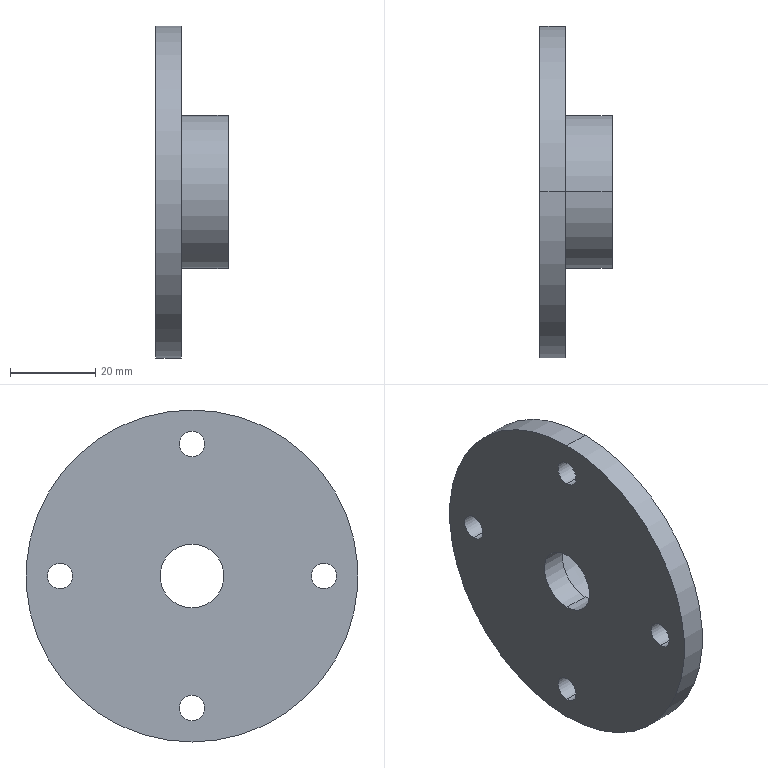Part | NX | features BREP 1 | 1 solid | 20 faces | box 17 x 78 x 78 mm | volume 31804 mm3 | cylinder 14 | plane 4 | cone 2 | commonest cylinder face diameters 6 x8 15 x2 36 x2 78 x2
STEP:
#1=CARTESIAN_POINT('',(6.,0.,-28.));
#2=VERTEX_POINT('',#1);
#3=CARTESIAN_POINT('',(6.,0.,-34.));
#4=VERTEX_POINT('',#3);
#5=CARTESIAN_POINT('',(6.,0.,-31.));
#6=DIRECTION('',(1.,0.,0.));
#7=DIRECTION('',(0.,0.,1.));
#8=AXIS2_PLACEMENT_3D('',#5,#6,#7);
#9=CIRCLE('',#8,3.);
#10=EDGE_CURVE('',#2,#4,#9,.T.);
#11=ORIENTED_EDGE('',*,*,#10,.T.);
#12=CARTESIAN_POINT('',(0.,0.,-34.));
#13=VERTEX_POINT('',#12);
#14=CARTESIAN_POINT('',(17.001,0.,-34.));
#15=DIRECTION('',(-1.,0.,0.));
#16=VECTOR('',#15,1000.);
#17=LINE('',#14,#16);
#18=EDGE_CURVE('',#4,#13,#17,.T.);
#19=ORIENTED_EDGE('',*,*,#18,.T.);
#20=CARTESIAN_POINT('',(0.,0.,-28.));
#21=VERTEX_POINT('',#20);
#22=CARTESIAN_POINT('',(0.,0.,-31.));
#23=DIRECTION('',(-1.,0.,0.));
#24=DIRECTION('',(0.,0.,1.));
#25=AXIS2_PLACEMENT_3D('',#22,#23,#24);
#26=CIRCLE('',#25,3.);
#27=EDGE_CURVE('',#13,#21,#26,.T.);
#28=ORIENTED_EDGE('',*,*,#27,.T.);
#29=CARTESIAN_POINT('',(17.001,0.,-28.));
#30=DIRECTION('',(-1.,0.,0.));
#31=VECTOR('',#30,1000.);
#32=LINE('',#29,#31);
#33=EDGE_CURVE('',#2,#21,#32,.T.);
#34=ORIENTED_EDGE('',*,*,#33,.F.);
#35=EDGE_LOOP('',(#11,#19,#28,#34));
#36=FACE_BOUND('',#35,.T.);
#37=CARTESIAN_POINT('',(17.001,0.,-31.));
#38=DIRECTION('',(-1.,0.,0.));
#39=DIRECTION('',(0.,0.,-1.));
#40=AXIS2_PLACEMENT_3D('',#37,#38,#39);
#41=CYLINDRICAL_SURFACE('',#40,3.);
#42=ADVANCED_FACE('',(#36),#41,.F.);
#43=CARTESIAN_POINT('',(6.,-31.,3.));
#44=VERTEX_POINT('',#43);
#45=CARTESIAN_POINT('',(6.,-31.,-3.));
#46=VERTEX_POINT('',#45);
#47=CARTESIAN_POINT('',(6.,-31.,0.));
#48=DIRECTION('',(1.,0.,0.));
#49=DIRECTION('',(0.,0.,1.));
#50=AXIS2_PLACEMENT_3D('',#47,#48,#49);
#51=CIRCLE('',#50,3.);
#52=EDGE_CURVE('',#44,#46,#51,.T.);
#53=ORIENTED_EDGE('',*,*,#52,.T.);
#54=CARTESIAN_POINT('',(0.,-31.,-3.));
#55=VERTEX_POINT('',#54);
#56=CARTESIAN_POINT('',(17.001,-31.,-3.));
#57=DIRECTION('',(-1.,0.,0.));
#58=VECTOR('',#57,1000.);
#59=LINE('',#56,#58);
#60=EDGE_CURVE('',#46,#55,#59,.T.);
#61=ORIENTED_EDGE('',*,*,#60,.T.);
#62=CARTESIAN_POINT('',(0.,-31.,3.));
#63=VERTEX_POINT('',#62);
#64=CARTESIAN_POINT('',(0.,-31.,0.));
#65=DIRECTION('',(-1.,0.,0.));
#66=DIRECTION('',(0.,0.,1.));
#67=AXIS2_PLACEMENT_3D('',#64,#65,#66);
#68=CIRCLE('',#67,3.);
#69=EDGE_CURVE('',#55,#63,#68,.T.);
#70=ORIENTED_EDGE('',*,*,#69,.T.);
#71=CARTESIAN_POINT('',(17.001,-31.,3.));
#72=DIRECTION('',(-1.,0.,0.));
#73=VECTOR('',#72,1000.);
#74=LINE('',#71,#73);
#75=EDGE_CURVE('',#44,#63,#74,.T.);
#76=ORIENTED_EDGE('',*,*,#75,.F.);
#77=EDGE_LOOP('',(#53,#61,#70,#76));
#78=FACE_BOUND('',#77,.T.);
#79=CARTESIAN_POINT('',(17.001,-31.,0.));
#80=DIRECTION('',(-1.,0.,0.));
#81=DIRECTION('',(0.,0.,-1.));
#82=AXIS2_PLACEMENT_3D('',#79,#80,#81);
#83=CYLINDRICAL_SURFACE('',#82,3.);
#84=ADVANCED_FACE('',(#78),#83,.F.);
#85=CARTESIAN_POINT('',(6.,0.,34.));
#86=VERTEX_POINT('',#85);
#87=CARTESIAN_POINT('',(6.,0.,28.));
#88=VERTEX_POINT('',#87);
#89=CARTESIAN_POINT('',(6.,0.,31.));
#90=DIRECTION('',(1.,0.,0.));
#91=DIRECTION('',(0.,0.,1.));
#92=AXIS2_PLACEMENT_3D('',#89,#90,#91);
#93=CIRCLE('',#92,3.);
#94=EDGE_CURVE('',#86,#88,#93,.T.);
#95=ORIENTED_EDGE('',*,*,#94,.T.);
#96=CARTESIAN_POINT('',(0.,0.,28.));
#97=VERTEX_POINT('',#96);
#98=CARTESIAN_POINT('',(17.001,0.,28.));
#99=DIRECTION('',(-1.,0.,0.));
#100=VECTOR('',#99,1000.);
#101=LINE('',#98,#100);
#102=EDGE_CURVE('',#88,#97,#101,.T.);
#103=ORIENTED_EDGE('',*,*,#102,.T.);
#104=CARTESIAN_POINT('',(0.,0.,34.));
#105=VERTEX_POINT('',#104);
#106=CARTESIAN_POINT('',(0.,0.,31.));
#107=DIRECTION('',(-1.,0.,0.));
#108=DIRECTION('',(0.,0.,1.));
#109=AXIS2_PLACEMENT_3D('',#106,#107,#108);
#110=CIRCLE('',#109,3.);
#111=EDGE_CURVE('',#97,#105,#110,.T.);
#112=ORIENTED_EDGE('',*,*,#111,.T.);
#113=CARTESIAN_POINT('',(17.001,0.,34.));
#114=DIRECTION('',(-1.,0.,0.));
#115=VECTOR('',#114,1000.);
#116=LINE('',#113,#115);
#117=EDGE_CURVE('',#86,#105,#116,.T.);
#118=ORIENTED_EDGE('',*,*,#117,.F.);
#119=EDGE_LOOP('',(#95,#103,#112,#118));
#120=FACE_BOUND('',#119,.T.);
#121=CARTESIAN_POINT('',(17.001,0.,31.));
#122=DIRECTION('',(-1.,0.,0.));
#123=DIRECTION('',(0.,0.,-1.));
#124=AXIS2_PLACEMENT_3D('',#121,#122,#123);
#125=CYLINDRICAL_SURFACE('',#124,3.);
#126=ADVANCED_FACE('',(#120),#125,.F.);
#127=CARTESIAN_POINT('',(6.,31.,3.));
#128=VERTEX_POINT('',#127);
#129=CARTESIAN_POINT('',(6.,31.,-3.));
#130=VERTEX_POINT('',#129);
#131=CARTESIAN_POINT('',(6.,31.,0.));
#132=DIRECTION('',(1.,0.,0.));
#133=DIRECTION('',(0.,0.,1.));
#134=AXIS2_PLACEMENT_3D('',#131,#132,#133);
#135=CIRCLE('',#134,3.);
#136=EDGE_CURVE('',#128,#130,#135,.T.);
#137=ORIENTED_EDGE('',*,*,#136,.T.);
#138=CARTESIAN_POINT('',(0.,31.,-3.));
#139=VERTEX_POINT('',#138);
#140=CARTESIAN_POINT('',(17.001,31.,-3.));
#141=DIRECTION('',(-1.,0.,0.));
#142=VECTOR('',#141,1000.);
#143=LINE('',#140,#142);
#144=EDGE_CURVE('',#130,#139,#143,.T.);
#145=ORIENTED_EDGE('',*,*,#144,.T.);
#146=CARTESIAN_POINT('',(0.,31.,3.));
#147=VERTEX_POINT('',#146);
#148=CARTESIAN_POINT('',(0.,31.,0.));
#149=DIRECTION('',(-1.,0.,0.));
#150=DIRECTION('',(0.,0.,1.));
#151=AXIS2_PLACEMENT_3D('',#148,#149,#150);
#152=CIRCLE('',#151,3.);
#153=EDGE_CURVE('',#139,#147,#152,.T.);
#154=ORIENTED_EDGE('',*,*,#153,.T.);
#155=CARTESIAN_POINT('',(17.001,31.,3.));
#156=DIRECTION('',(-1.,0.,0.));
#157=VECTOR('',#156,1000.);
#158=LINE('',#155,#157);
#159=EDGE_CURVE('',#128,#147,#158,.T.);
#160=ORIENTED_EDGE('',*,*,#159,.F.);
#161=EDGE_LOOP('',(#137,#145,#154,#160));
#162=FACE_BOUND('',#161,.T.);
#163=CARTESIAN_POINT('',(17.001,31.,0.));
#164=DIRECTION('',(-1.,0.,0.));
#165=DIRECTION('',(0.,0.,-1.));
#166=AXIS2_PLACEMENT_3D('',#163,#164,#165);
#167=CYLINDRICAL_SURFACE('',#166,3.);
#168=ADVANCED_FACE('',(#162),#167,.F.);
#169=CARTESIAN_POINT('',(6.,0.,-12.));
#170=VERTEX_POINT('',#169);
#171=CARTESIAN_POINT('',(6.,0.,12.));
#172=VERTEX_POINT('',#171);
#173=CARTESIAN_POINT('',(6.,0.,0.));
#174=DIRECTION('',(-1.,0.,0.));
#175=DIRECTION('',(0.,0.,1.));
#176=AXIS2_PLACEMENT_3D('',#173,#174,#175);
#177=CIRCLE('',#176,12.);
#178=EDGE_CURVE('',#170,#172,#177,.T.);
#179=ORIENTED_EDGE('',*,*,#178,.T.);
#180=CARTESIAN_POINT('',(17.,0.,15.));
#181=VERTEX_POINT('',#180);
#182=CARTESIAN_POINT('',(6.,0.,12.));
#183=DIRECTION('',(0.9648,0.,0.2631));
#184=VECTOR('',#183,1000.);
#185=LINE('',#182,#184);
#186=EDGE_CURVE('',#181,#172,#185,.F.);
#187=ORIENTED_EDGE('',*,*,#186,.F.);
#188=CARTESIAN_POINT('',(17.,0.,-15.));
#189=VERTEX_POINT('',#188);
#190=CARTESIAN_POINT('',(17.,0.,0.));
#191=DIRECTION('',(-1.,0.,0.));
#192=DIRECTION('',(0.,0.,1.));
#193=AXIS2_PLACEMENT_3D('',#190,#191,#192);
#194=CIRCLE('',#193,15.);
#195=EDGE_CURVE('',#189,#181,#194,.T.);
#196=ORIENTED_EDGE('',*,*,#195,.F.);
#197=CARTESIAN_POINT('',(6.,0.,-12.));
#198=DIRECTION('',(0.9648,0.,-0.2631));
#199=VECTOR('',#198,1000.);
#200=LINE('',#197,#199);
#201=EDGE_CURVE('',#189,#170,#200,.F.);
#202=ORIENTED_EDGE('',*,*,#201,.T.);
#203=EDGE_LOOP('',(#179,#187,#196,#202));
#204=FACE_BOUND('',#203,.T.);
#205=CARTESIAN_POINT('',(6.,0.,0.));
#206=DIRECTION('',(1.,0.,0.));
#207=DIRECTION('',(0.,0.,1.));
#208=AXIS2_PLACEMENT_3D('',#205,#206,#207);
#209=CONICAL_SURFACE('',#208,12.,0.2663);
#210=ADVANCED_FACE('',(#204),#209,.F.);
#211=CARTESIAN_POINT('',(17.,0.,18.));
#212=VERTEX_POINT('',#211);
#213=CARTESIAN_POINT('',(17.,0.,-18.));
#214=VERTEX_POINT('',#213);
#215=CARTESIAN_POINT('',(17.,0.,0.));
#216=DIRECTION('',(-1.,0.,0.));
#217=DIRECTION('',(0.,0.,1.));
#218=AXIS2_PLACEMENT_3D('',#215,#216,#217);
#219=CIRCLE('',#218,18.);
#220=EDGE_CURVE('',#212,#214,#219,.T.);
#221=ORIENTED_EDGE('',*,*,#220,.T.);
#222=CARTESIAN_POINT('',(6.,0.,-18.));
#223=VERTEX_POINT('',#222);
#224=CARTESIAN_POINT('',(6.,0.,-18.));
#225=DIRECTION('',(-1.,0.,0.));
#226=VECTOR('',#225,1000.);
#227=LINE('',#224,#226);
#228=EDGE_CURVE('',#214,#223,#227,.T.);
#229=ORIENTED_EDGE('',*,*,#228,.T.);
#230=CARTESIAN_POINT('',(6.,0.,18.));
#231=VERTEX_POINT('',#230);
#232=CARTESIAN_POINT('',(6.,0.,0.));
#233=DIRECTION('',(-1.,0.,0.));
#234=DIRECTION('',(0.,0.,1.));
#235=AXIS2_PLACEMENT_3D('',#232,#233,#234);
#236=CIRCLE('',#235,18.);
#237=EDGE_CURVE('',#231,#223,#236,.T.);
#238=ORIENTED_EDGE('',*,*,#237,.F.);
#239=CARTESIAN_POINT('',(6.,0.,18.));
#240=DIRECTION('',(-1.,0.,0.));
#241=VECTOR('',#240,1000.);
#242=LINE('',#239,#241);
#243=EDGE_CURVE('',#212,#231,#242,.T.);
#244=ORIENTED_EDGE('',*,*,#243,.F.);
#245=EDGE_LOOP('',(#221,#229,#238,#244));
#246=FACE_BOUND('',#245,.T.);
#247=CARTESIAN_POINT('',(6.,0.,0.));
#248=DIRECTION('',(-1.,0.,0.));
#249=DIRECTION('',(0.,0.,-1.));
#250=AXIS2_PLACEMENT_3D('',#247,#248,#249);
#251=CYLINDRICAL_SURFACE('',#250,18.);
#252=ADVANCED_FACE('',(#246),#251,.T.);
#253=CARTESIAN_POINT('',(6.,0.,39.));
#254=VERTEX_POINT('',#253);
#255=CARTESIAN_POINT('',(6.,0.,-39.));
#256=VERTEX_POINT('',#255);
#257=CARTESIAN_POINT('',(6.,0.,0.));
#258=DIRECTION('',(-1.,0.,0.));
#259=DIRECTION('',(0.,0.,1.));
#260=AXIS2_PLACEMENT_3D('',#257,#258,#259);
#261=CIRCLE('',#260,39.);
#262=EDGE_CURVE('',#254,#256,#261,.T.);
#263=ORIENTED_EDGE('',*,*,#262,.T.);
#264=CARTESIAN_POINT('',(0.,0.,-39.));
#265=VERTEX_POINT('',#264);
#266=CARTESIAN_POINT('',(6.,0.,-39.));
#267=DIRECTION('',(-1.,0.,0.));
#268=VECTOR('',#267,1000.);
#269=LINE('',#266,#268);
#270=EDGE_CURVE('',#256,#265,#269,.T.);
#271=ORIENTED_EDGE('',*,*,#270,.T.);
#272=CARTESIAN_POINT('',(0.,0.,39.));
#273=VERTEX_POINT('',#272);
#274=CARTESIAN_POINT('',(0.,0.,0.));
#275=DIRECTION('',(-1.,0.,0.));
#276=DIRECTION('',(0.,0.,1.));
#277=AXIS2_PLACEMENT_3D('',#274,#275,#276);
#278=CIRCLE('',#277,39.);
#279=EDGE_CURVE('',#273,#265,#278,.T.);
#280=ORIENTED_EDGE('',*,*,#279,.F.);
#281=CARTESIAN_POINT('',(6.,0.,39.));
#282=DIRECTION('',(-1.,0.,0.));
#283=VECTOR('',#282,1000.);
#284=LINE('',#281,#283);
#285=EDGE_CURVE('',#254,#273,#284,.T.);
#286=ORIENTED_EDGE('',*,*,#285,.F.);
#287=EDGE_LOOP('',(#263,#271,#280,#286));
#288=FACE_BOUND('',#287,.T.);
#289=CARTESIAN_POINT('',(6.,0.,0.));
#290=DIRECTION('',(-1.,0.,0.));
#291=DIRECTION('',(0.,0.,-1.));
#292=AXIS2_PLACEMENT_3D('',#289,#290,#291);
#293=CYLINDRICAL_SURFACE('',#292,39.);
#294=ADVANCED_FACE('',(#288),#293,.T.);
#295=CARTESIAN_POINT('',(6.,0.,-7.5));
#296=VERTEX_POINT('',#295);
#297=CARTESIAN_POINT('',(6.,0.,7.5));
#298=VERTEX_POINT('',#297);
#299=CARTESIAN_POINT('',(6.,0.,0.));
#300=DIRECTION('',(-1.,0.,0.));
#301=DIRECTION('',(0.,0.,1.));
#302=AXIS2_PLACEMENT_3D('',#299,#300,#301);
#303=CIRCLE('',#302,7.5);
#304=EDGE_CURVE('',#296,#298,#303,.T.);
#305=ORIENTED_EDGE('',*,*,#304,.F.);
#306=CARTESIAN_POINT('',(0.,0.,-7.5));
#307=VERTEX_POINT('',#306);
#308=CARTESIAN_POINT('',(6.,0.,-7.5));
#309=DIRECTION('',(-1.,0.,0.));
#310=VECTOR('',#309,1000.);
#311=LINE('',#308,#310);
#312=EDGE_CURVE('',#296,#307,#311,.T.);
#313=ORIENTED_EDGE('',*,*,#312,.T.);
#314=CARTESIAN_POINT('',(0.,0.,7.5));
#315=VERTEX_POINT('',#314);
#316=CARTESIAN_POINT('',(0.,0.,0.));
#317=DIRECTION('',(-1.,0.,0.));
#318=DIRECTION('',(0.,0.,1.));
#319=AXIS2_PLACEMENT_3D('',#316,#317,#318);
#320=CIRCLE('',#319,7.5);
#321=EDGE_CURVE('',#307,#315,#320,.T.);
#322=ORIENTED_EDGE('',*,*,#321,.T.);
#323=CARTESIAN_POINT('',(6.,0.,7.5));
#324=DIRECTION('',(-1.,0.,0.));
#325=VECTOR('',#324,1000.);
#326=LINE('',#323,#325);
#327=EDGE_CURVE('',#298,#315,#326,.T.);
#328=ORIENTED_EDGE('',*,*,#327,.F.);
#329=EDGE_LOOP('',(#305,#313,#322,#328));
#330=FACE_BOUND('',#329,.T.);
#331=CARTESIAN_POINT('',(6.,0.,0.));
#332=DIRECTION('',(-1.,0.,0.));
#333=DIRECTION('',(0.,0.,-1.));
#334=AXIS2_PLACEMENT_3D('',#331,#332,#333);
#335=CYLINDRICAL_SURFACE('',#334,7.5);
#336=ADVANCED_FACE('',(#330),#335,.F.);
#337=ORIENTED_EDGE('',*,*,#312,.F.);
#338=CARTESIAN_POINT('',(6.,0.,0.));
#339=DIRECTION('',(-1.,0.,0.));
#340=DIRECTION('',(0.,0.,1.));
#341=AXIS2_PLACEMENT_3D('',#338,#339,#340);
#342=CIRCLE('',#341,7.5);
#343=EDGE_CURVE('',#298,#296,#342,.T.);
#344=ORIENTED_EDGE('',*,*,#343,.F.);
#345=ORIENTED_EDGE('',*,*,#327,.T.);
#346=CARTESIAN_POINT('',(0.,0.,0.));
#347=DIRECTION('',(-1.,0.,0.));
#348=DIRECTION('',(0.,0.,1.));
#349=AXIS2_PLACEMENT_3D('',#346,#347,#348);
#350=CIRCLE('',#349,7.5);
#351=EDGE_CURVE('',#315,#307,#350,.T.);
#352=ORIENTED_EDGE('',*,*,#351,.T.);
#353=EDGE_LOOP('',(#337,#344,#345,#352));
#354=FACE_BOUND('',#353,.T.);
#355=CARTESIAN_POINT('',(6.,0.,0.));
#356=DIRECTION('',(-1.,0.,0.));
#357=DIRECTION('',(0.,0.,-1.));
#358=AXIS2_PLACEMENT_3D('',#355,#356,#357);
#359=CYLINDRICAL_SURFACE('',#358,7.5);
#360=ADVANCED_FACE('',(#354),#359,.F.);
#361=ORIENTED_EDGE('',*,*,#279,.T.);
#362=CARTESIAN_POINT('',(0.,0.,0.));
#363=DIRECTION('',(-1.,0.,0.));
#364=DIRECTION('',(0.,0.,1.));
#365=AXIS2_PLACEMENT_3D('',#362,#363,#364);
#366=CIRCLE('',#365,39.);
#367=EDGE_CURVE('',#265,#273,#366,.T.);
#368=ORIENTED_EDGE('',*,*,#367,.T.);
#369=EDGE_LOOP('',(#361,#368));
#370=FACE_BOUND('',#369,.T.);
#371=CARTESIAN_POINT('',(0.,0.,-31.));
#372=DIRECTION('',(-1.,0.,0.));
#373=DIRECTION('',(0.,0.,1.));
#374=AXIS2_PLACEMENT_3D('',#371,#372,#373);
#375=CIRCLE('',#374,3.);
#376=EDGE_CURVE('',#21,#13,#375,.T.);
#377=ORIENTED_EDGE('',*,*,#376,.F.);
#378=ORIENTED_EDGE('',*,*,#27,.F.);
#379=EDGE_LOOP('',(#377,#378));
#380=FACE_BOUND('',#379,.T.);
#381=CARTESIAN_POINT('',(0.,-31.,0.));
#382=DIRECTION('',(-1.,0.,0.));
#383=DIRECTION('',(0.,0.,1.));
#384=AXIS2_PLACEMENT_3D('',#381,#382,#383);
#385=CIRCLE('',#384,3.);
#386=EDGE_CURVE('',#63,#55,#385,.T.);
#387=ORIENTED_EDGE('',*,*,#386,.F.);
#388=ORIENTED_EDGE('',*,*,#69,.F.);
#389=EDGE_LOOP('',(#387,#388));
#390=FACE_BOUND('',#389,.T.);
#391=CARTESIAN_POINT('',(0.,0.,31.));
#392=DIRECTION('',(-1.,0.,0.));
#393=DIRECTION('',(0.,0.,1.));
#394=AXIS2_PLACEMENT_3D('',#391,#392,#393);
#395=CIRCLE('',#394,3.);
#396=EDGE_CURVE('',#105,#97,#395,.T.);
#397=ORIENTED_EDGE('',*,*,#396,.F.);
#398=ORIENTED_EDGE('',*,*,#111,.F.);
#399=EDGE_LOOP('',(#397,#398));
#400=FACE_BOUND('',#399,.T.);
#401=CARTESIAN_POINT('',(0.,31.,0.));
#402=DIRECTION('',(-1.,0.,0.));
#403=DIRECTION('',(0.,0.,1.));
#404=AXIS2_PLACEMENT_3D('',#401,#402,#403);
#405=CIRCLE('',#404,3.);
#406=EDGE_CURVE('',#147,#139,#405,.T.);
#407=ORIENTED_EDGE('',*,*,#406,.F.);
#408=ORIENTED_EDGE('',*,*,#153,.F.);
#409=EDGE_LOOP('',(#407,#408));
#410=FACE_BOUND('',#409,.T.);
#411=ORIENTED_EDGE('',*,*,#351,.F.);
#412=ORIENTED_EDGE('',*,*,#321,.F.);
#413=EDGE_LOOP('',(#411,#412));
#414=FACE_BOUND('',#413,.T.);
#415=CARTESIAN_POINT('',(0.,7.5,0.));
#416=DIRECTION('',(1.,0.,0.));
#417=DIRECTION('',(0.,0.,1.));
#418=AXIS2_PLACEMENT_3D('',#415,#416,#417);
#419=PLANE('',#418);
#420=ADVANCED_FACE('',(#370,#380,#390,#400,#410,#414),#419,.F.);
#421=ORIENTED_EDGE('',*,*,#270,.F.);
#422=CARTESIAN_POINT('',(6.,0.,0.));
#423=DIRECTION('',(-1.,0.,0.));
#424=DIRECTION('',(0.,0.,1.));
#425=AXIS2_PLACEMENT_3D('',#422,#423,#424);
#426=CIRCLE('',#425,39.);
#427=EDGE_CURVE('',#256,#254,#426,.T.);
#428=ORIENTED_EDGE('',*,*,#427,.T.);
#429=ORIENTED_EDGE('',*,*,#285,.T.);
#430=ORIENTED_EDGE('',*,*,#367,.F.);
#431=EDGE_LOOP('',(#421,#428,#429,#430));
#432=FACE_BOUND('',#431,.T.);
#433=CARTESIAN_POINT('',(6.,0.,0.));
#434=DIRECTION('',(-1.,0.,0.));
#435=DIRECTION('',(0.,0.,-1.));
#436=AXIS2_PLACEMENT_3D('',#433,#434,#435);
#437=CYLINDRICAL_SURFACE('',#436,39.);
#438=ADVANCED_FACE('',(#432),#437,.T.);
#439=ORIENTED_EDGE('',*,*,#262,.F.);
#440=ORIENTED_EDGE('',*,*,#427,.F.);
#441=EDGE_LOOP('',(#439,#440));
#442=FACE_BOUND('',#441,.T.);
#443=ORIENTED_EDGE('',*,*,#10,.F.);
#444=CARTESIAN_POINT('',(6.,0.,-31.));
#445=DIRECTION('',(1.,0.,0.));
#446=DIRECTION('',(0.,0.,1.));
#447=AXIS2_PLACEMENT_3D('',#444,#445,#446);
#448=CIRCLE('',#447,3.);
#449=EDGE_CURVE('',#4,#2,#448,.T.);
#450=ORIENTED_EDGE('',*,*,#449,.F.);
#451=EDGE_LOOP('',(#443,#450));
#452=FACE_BOUND('',#451,.T.);
#453=ORIENTED_EDGE('',*,*,#52,.F.);
#454=CARTESIAN_POINT('',(6.,-31.,0.));
#455=DIRECTION('',(1.,0.,0.));
#456=DIRECTION('',(0.,0.,1.));
#457=AXIS2_PLACEMENT_3D('',#454,#455,#456);
#458=CIRCLE('',#457,3.);
#459=EDGE_CURVE('',#46,#44,#458,.T.);
#460=ORIENTED_EDGE('',*,*,#459,.F.);
#461=EDGE_LOOP('',(#453,#460));
#462=FACE_BOUND('',#461,.T.);
#463=ORIENTED_EDGE('',*,*,#94,.F.);
#464=CARTESIAN_POINT('',(6.,0.,31.));
#465=DIRECTION('',(1.,0.,0.));
#466=DIRECTION('',(0.,0.,1.));
#467=AXIS2_PLACEMENT_3D('',#464,#465,#466);
#468=CIRCLE('',#467,3.);
#469=EDGE_CURVE('',#88,#86,#468,.T.);
#470=ORIENTED_EDGE('',*,*,#469,.F.);
#471=EDGE_LOOP('',(#463,#470));
#472=FACE_BOUND('',#471,.T.);
#473=ORIENTED_EDGE('',*,*,#136,.F.);
#474=CARTESIAN_POINT('',(6.,31.,0.));
#475=DIRECTION('',(1.,0.,0.));
#476=DIRECTION('',(0.,0.,1.));
#477=AXIS2_PLACEMENT_3D('',#474,#475,#476);
#478=CIRCLE('',#477,3.);
#479=EDGE_CURVE('',#130,#128,#478,.T.);
#480=ORIENTED_EDGE('',*,*,#479,.F.);
#481=EDGE_LOOP('',(#473,#480));
#482=FACE_BOUND('',#481,.T.);
#483=ORIENTED_EDGE('',*,*,#237,.T.);
#484=CARTESIAN_POINT('',(6.,0.,0.));
#485=DIRECTION('',(-1.,0.,0.));
#486=DIRECTION('',(0.,0.,1.));
#487=AXIS2_PLACEMENT_3D('',#484,#485,#486);
#488=CIRCLE('',#487,18.);
#489=EDGE_CURVE('',#223,#231,#488,.T.);
#490=ORIENTED_EDGE('',*,*,#489,.T.);
#491=EDGE_LOOP('',(#483,#490));
#492=FACE_BOUND('',#491,.T.);
#493=CARTESIAN_POINT('',(6.,39.,0.));
#494=DIRECTION('',(-1.,0.,0.));
#495=DIRECTION('',(0.,-1.,0.));
#496=AXIS2_PLACEMENT_3D('',#493,#494,#495);
#497=PLANE('',#496);
#498=ADVANCED_FACE('',(#442,#452,#462,#472,#482,#492),#497,.F.);
#499=ORIENTED_EDGE('',*,*,#228,.F.);
#500=CARTESIAN_POINT('',(17.,0.,0.));
#501=DIRECTION('',(-1.,0.,0.));
#502=DIRECTION('',(0.,0.,1.));
#503=AXIS2_PLACEMENT_3D('',#500,#501,#502);
#504=CIRCLE('',#503,18.);
#505=EDGE_CURVE('',#214,#212,#504,.T.);
#506=ORIENTED_EDGE('',*,*,#505,.T.);
#507=ORIENTED_EDGE('',*,*,#243,.T.);
#508=ORIENTED_EDGE('',*,*,#489,.F.);
#509=EDGE_LOOP('',(#499,#506,#507,#508));
#510=FACE_BOUND('',#509,.T.);
#511=CARTESIAN_POINT('',(6.,0.,0.));
#512=DIRECTION('',(-1.,0.,0.));
#513=DIRECTION('',(0.,0.,-1.));
#514=AXIS2_PLACEMENT_3D('',#511,#512,#513);
#515=CYLINDRICAL_SURFACE('',#514,18.);
#516=ADVANCED_FACE('',(#510),#515,.T.);
#517=ORIENTED_EDGE('',*,*,#220,.F.);
#518=ORIENTED_EDGE('',*,*,#505,.F.);
#519=EDGE_LOOP('',(#517,#518));
#520=FACE_BOUND('',#519,.T.);
#521=ORIENTED_EDGE('',*,*,#195,.T.);
#522=CARTESIAN_POINT('',(17.,0.,0.));
#523=DIRECTION('',(-1.,0.,0.));
#524=DIRECTION('',(0.,0.,1.));
#525=AXIS2_PLACEMENT_3D('',#522,#523,#524);
#526=CIRCLE('',#525,15.);
#527=EDGE_CURVE('',#181,#189,#526,.T.);
#528=ORIENTED_EDGE('',*,*,#527,.T.);
#529=EDGE_LOOP('',(#521,#528));
#530=FACE_BOUND('',#529,.T.);
#531=CARTESIAN_POINT('',(17.,18.,0.));
#532=DIRECTION('',(-1.,0.,0.));
#533=DIRECTION('',(0.,-1.,0.));
#534=AXIS2_PLACEMENT_3D('',#531,#532,#533);
#535=PLANE('',#534);
#536=ADVANCED_FACE('',(#520,#530),#535,.F.);
#537=ORIENTED_EDGE('',*,*,#186,.T.);
#538=CARTESIAN_POINT('',(6.,0.,0.));
#539=DIRECTION('',(-1.,0.,0.));
#540=DIRECTION('',(0.,0.,1.));
#541=AXIS2_PLACEMENT_3D('',#538,#539,#540);
#542=CIRCLE('',#541,12.);
#543=EDGE_CURVE('',#172,#170,#542,.T.);
#544=ORIENTED_EDGE('',*,*,#543,.T.);
#545=ORIENTED_EDGE('',*,*,#201,.F.);
#546=ORIENTED_EDGE('',*,*,#527,.F.);
#547=EDGE_LOOP('',(#537,#544,#545,#546));
#548=FACE_BOUND('',#547,.T.);
#549=CARTESIAN_POINT('',(6.,0.,0.));
#550=DIRECTION('',(1.,0.,0.));
#551=DIRECTION('',(0.,0.,1.));
#552=AXIS2_PLACEMENT_3D('',#549,#550,#551);
#553=CONICAL_SURFACE('',#552,12.,0.2663);
#554=ADVANCED_FACE('',(#548),#553,.F.);
#555=ORIENTED_EDGE('',*,*,#178,.F.);
#556=ORIENTED_EDGE('',*,*,#543,.F.);
#557=EDGE_LOOP('',(#555,#556));
#558=FACE_BOUND('',#557,.T.);
#559=ORIENTED_EDGE('',*,*,#343,.T.);
#560=ORIENTED_EDGE('',*,*,#304,.T.);
#561=EDGE_LOOP('',(#559,#560));
#562=FACE_BOUND('',#561,.T.);
#563=CARTESIAN_POINT('',(6.,12.,0.));
#564=DIRECTION('',(-1.,0.,0.));
#565=DIRECTION('',(0.,-1.,0.));
#566=AXIS2_PLACEMENT_3D('',#563,#564,#565);
#567=PLANE('',#566);
#568=ADVANCED_FACE('',(#558,#562),#567,.F.);
#569=ORIENTED_EDGE('',*,*,#144,.F.);
#570=ORIENTED_EDGE('',*,*,#479,.T.);
#571=ORIENTED_EDGE('',*,*,#159,.T.);
#572=ORIENTED_EDGE('',*,*,#406,.T.);
#573=EDGE_LOOP('',(#569,#570,#571,#572));
#574=FACE_BOUND('',#573,.T.);
#575=CARTESIAN_POINT('',(17.001,31.,0.));
#576=DIRECTION('',(-1.,0.,0.));
#577=DIRECTION('',(0.,0.,-1.));
#578=AXIS2_PLACEMENT_3D('',#575,#576,#577);
#579=CYLINDRICAL_SURFACE('',#578,3.);
#580=ADVANCED_FACE('',(#574),#579,.F.);
#581=ORIENTED_EDGE('',*,*,#102,.F.);
#582=ORIENTED_EDGE('',*,*,#469,.T.);
#583=ORIENTED_EDGE('',*,*,#117,.T.);
#584=ORIENTED_EDGE('',*,*,#396,.T.);
#585=EDGE_LOOP('',(#581,#582,#583,#584));
#586=FACE_BOUND('',#585,.T.);
#587=CARTESIAN_POINT('',(17.001,0.,31.));
#588=DIRECTION('',(-1.,0.,0.));
#589=DIRECTION('',(0.,0.,-1.));
#590=AXIS2_PLACEMENT_3D('',#587,#588,#589);
#591=CYLINDRICAL_SURFACE('',#590,3.);
#592=ADVANCED_FACE('',(#586),#591,.F.);
#593=ORIENTED_EDGE('',*,*,#60,.F.);
#594=ORIENTED_EDGE('',*,*,#459,.T.);
#595=ORIENTED_EDGE('',*,*,#75,.T.);
#596=ORIENTED_EDGE('',*,*,#386,.T.);
#597=EDGE_LOOP('',(#593,#594,#595,#596));
#598=FACE_BOUND('',#597,.T.);
#599=CARTESIAN_POINT('',(17.001,-31.,0.));
#600=DIRECTION('',(-1.,0.,0.));
#601=DIRECTION('',(0.,0.,-1.));
#602=AXIS2_PLACEMENT_3D('',#599,#600,#601);
#603=CYLINDRICAL_SURFACE('',#602,3.);
#604=ADVANCED_FACE('',(#598),#603,.F.);
#605=ORIENTED_EDGE('',*,*,#18,.F.);
#606=ORIENTED_EDGE('',*,*,#449,.T.);
#607=ORIENTED_EDGE('',*,*,#33,.T.);
#608=ORIENTED_EDGE('',*,*,#376,.T.);
#609=EDGE_LOOP('',(#605,#606,#607,#608));
#610=FACE_BOUND('',#609,.T.);
#611=CARTESIAN_POINT('',(17.001,0.,-31.));
#612=DIRECTION('',(-1.,0.,0.));
#613=DIRECTION('',(0.,0.,-1.));
#614=AXIS2_PLACEMENT_3D('',#611,#612,#613);
#615=CYLINDRICAL_SURFACE('',#614,3.);
#616=ADVANCED_FACE('',(#610),#615,.F.);
#617=CLOSED_SHELL('',(#42,#84,#126,#168,#210,#252,#294,#336,#360,#420,#438,#498,#516,#536,#554,#568,#580,#592,#604,#616));
#618=MANIFOLD_SOLID_BREP('',#617);
#619=(LENGTH_UNIT()NAMED_UNIT(*)SI_UNIT(.MILLI.,.METRE.));
#620=UNCERTAINTY_MEASURE_WITH_UNIT(LENGTH_MEASURE(0.00001),#619,'','');
#621=(NAMED_UNIT(*)PLANE_ANGLE_UNIT()SI_UNIT($,.RADIAN.));
#622=(NAMED_UNIT(*)SI_UNIT($,.STERADIAN.)SOLID_ANGLE_UNIT());
#623=(GEOMETRIC_REPRESENTATION_CONTEXT(3)GLOBAL_UNCERTAINTY_ASSIGNED_CONTEXT((#620))GLOBAL_UNIT_ASSIGNED_CONTEXT((#619,#621,#622))REPRESENTATION_CONTEXT('',''));
#624=ADVANCED_BREP_SHAPE_REPRESENTATION('',(#618),#623);